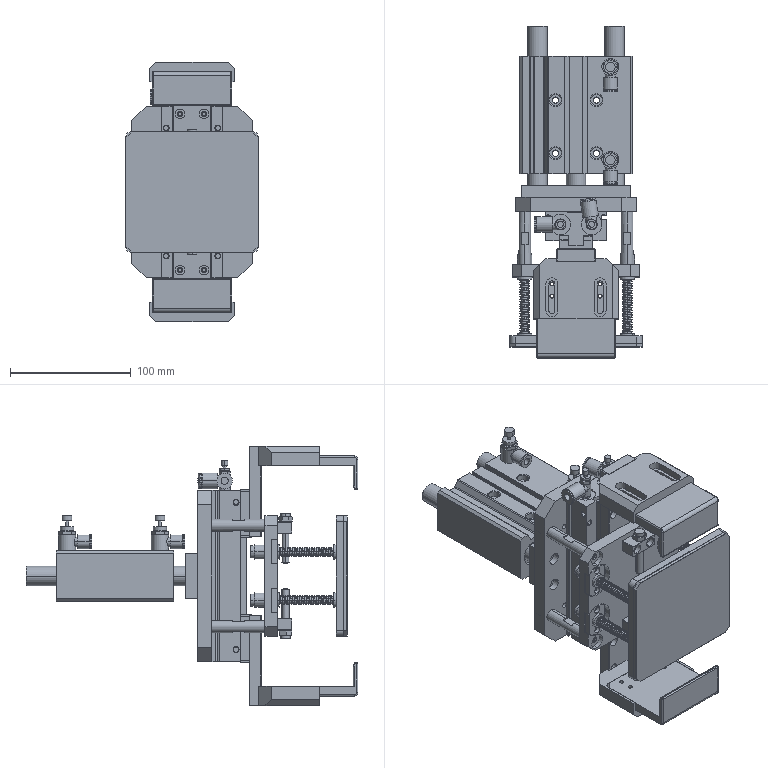Part | SolidWorks | features CompositeCurve 3 | 57 solids | 1884 faces | box 110 x 275 x 215 mm | volume 1117896 mm3 | cylinder 859 | plane 765 | cone 218 | torus 16 | spline 14 | sphere 12 | commonest cylinder face diameters 8 x84 10 x60 6 x50 12 x48 4 x45 3.3 x40